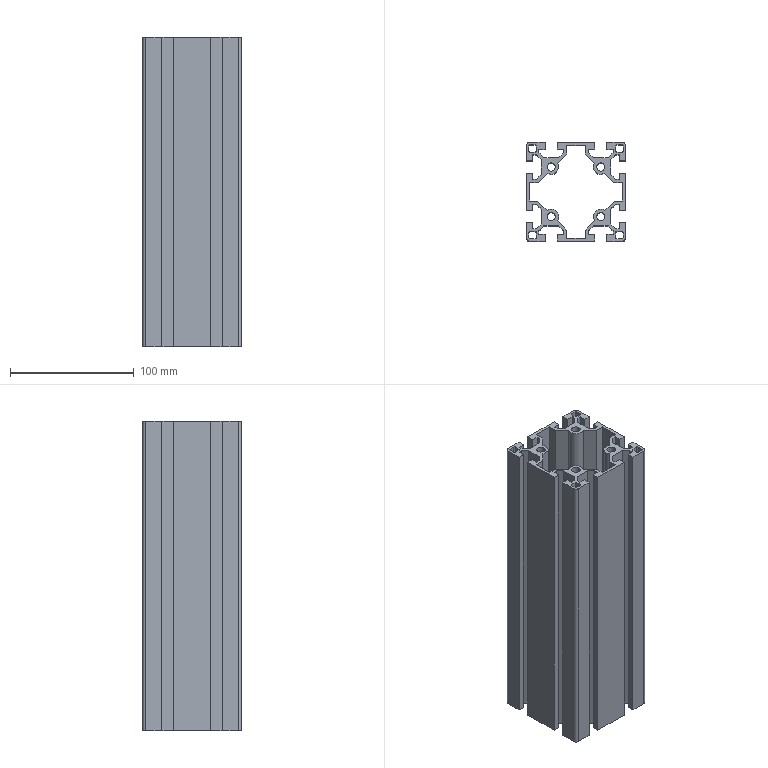Part | NX | 1 solid | 156 faces | box 80 x 80 x 250 mm | volume 438001 mm3 | plane 122 | cylinder 34 | commonest cylinder face diameters 2 x16 6.8 x8 11.8 x6 5.64 x4